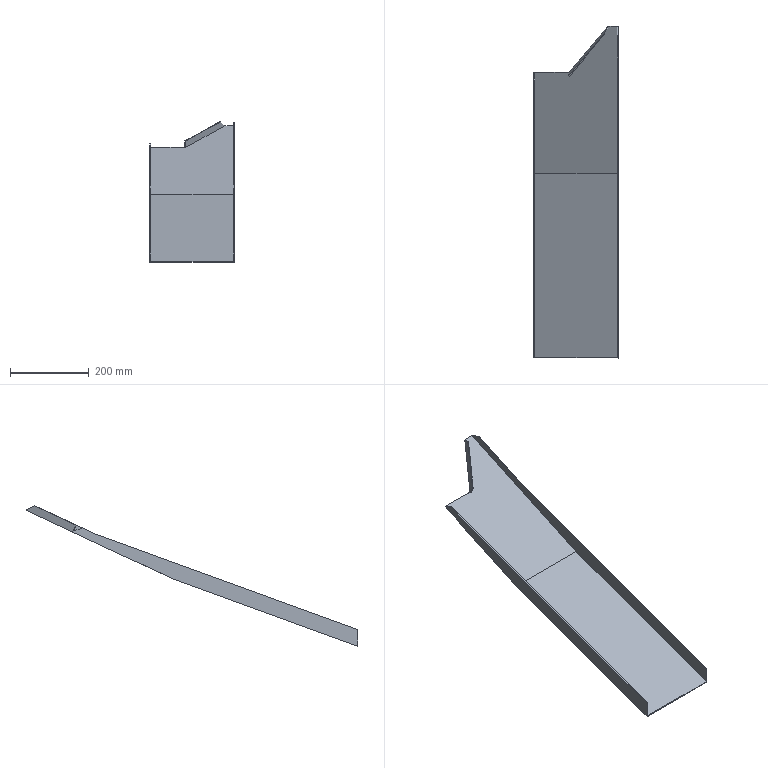Part | NX | features solid 2 | 1 solid | 26 faces | box 215.004 x 843.442 x 357.356 mm | volume 469723 mm3 | plane 26
STEP:
#1=CARTESIAN_POINT('',(-102.,-351.532,-337.023));
#2=VERTEX_POINT('',#1);
#3=CARTESIAN_POINT('',(-313.,-351.532,-337.004));
#4=VERTEX_POINT('',#3);
#5=CARTESIAN_POINT('',(-135.01,-351.532,-337.02));
#6=DIRECTION('',(1.,0.,-0.00008812));
#7=VECTOR('',#6,1000.);
#8=LINE('',#5,#7);
#9=EDGE_CURVE('',#2,#4,#8,.F.);
#10=ORIENTED_EDGE('',*,*,#9,.F.);
#11=CARTESIAN_POINT('',(-101.997,22.596,-162.564));
#12=VERTEX_POINT('',#11);
#13=CARTESIAN_POINT('',(-101.999,-191.108,-262.216));
#14=DIRECTION('',(0.000007217,0.9063,0.4226));
#15=VECTOR('',#14,1000.);
#16=LINE('',#13,#15);
#17=EDGE_CURVE('',#2,#12,#16,.T.);
#18=ORIENTED_EDGE('',*,*,#17,.T.);
#19=CARTESIAN_POINT('',(-126.636,22.592,-162.564));
#20=VERTEX_POINT('',#19);
#21=CARTESIAN_POINT('',(72.152,22.629,-162.564));
#22=DIRECTION('',(-1.,-0.000189,0.));
#23=VECTOR('',#22,1000.);
#24=LINE('',#21,#23);
#25=EDGE_CURVE('',#12,#20,#24,.T.);
#26=ORIENTED_EDGE('',*,*,#25,.T.);
#27=CARTESIAN_POINT('',(-125.044,21.495,-163.076));
#28=VERTEX_POINT('',#27);
#29=CARTESIAN_POINT('',(-18.326,-52.058,-197.383));
#30=DIRECTION('',(0.796,-0.5486,-0.2559));
#31=VECTOR('',#30,1000.);
#32=LINE('',#29,#31);
#33=EDGE_CURVE('',#28,#20,#32,.F.);
#34=ORIENTED_EDGE('',*,*,#33,.F.);
#35=CARTESIAN_POINT('',(-223.923,-96.344,-218.016));
#36=VERTEX_POINT('',#35);
#37=CARTESIAN_POINT('',(-241.722,-117.556,-227.906));
#38=DIRECTION('',(-0.6053,-0.7214,-0.3363));
#39=VECTOR('',#38,1000.);
#40=LINE('',#37,#39);
#41=EDGE_CURVE('',#28,#36,#40,.T.);
#42=ORIENTED_EDGE('',*,*,#41,.T.);
#43=CARTESIAN_POINT('',(-225.515,-95.247,-217.504));
#44=VERTEX_POINT('',#43);
#45=CARTESIAN_POINT('',(-117.204,-169.896,-252.323));
#46=DIRECTION('',(0.796,-0.5486,-0.2559));
#47=VECTOR('',#46,1000.);
#48=LINE('',#45,#47);
#49=EDGE_CURVE('',#44,#36,#48,.T.);
#50=ORIENTED_EDGE('',*,*,#49,.F.);
#51=CARTESIAN_POINT('',(-224.805,-94.402,-217.11));
#52=VERTEX_POINT('',#51);
#53=CARTESIAN_POINT('',(-243.314,-116.459,-227.394));
#54=DIRECTION('',(-0.6053,-0.7214,-0.3363));
#55=VECTOR('',#54,1000.);
#56=LINE('',#53,#55);
#57=EDGE_CURVE('',#52,#44,#56,.T.);
#58=ORIENTED_EDGE('',*,*,#57,.F.);
#59=CARTESIAN_POINT('',(-314.998,-94.419,-217.11));
#60=VERTEX_POINT('',#59);
#61=CARTESIAN_POINT('',(-135.022,-94.385,-217.11));
#62=DIRECTION('',(1.,0.000189,0.));
#63=VECTOR('',#62,1000.);
#64=LINE('',#61,#63);
#65=EDGE_CURVE('',#60,#52,#64,.T.);
#66=ORIENTED_EDGE('',*,*,#65,.F.);
#67=CARTESIAN_POINT('',(-314.998,-95.264,-217.504));
#68=VERTEX_POINT('',#67);
#69=CARTESIAN_POINT('',(-314.999,-191.114,-262.2));
#70=DIRECTION('',(0.000007217,0.9063,0.4226));
#71=VECTOR('',#70,1000.);
#72=LINE('',#69,#71);
#73=EDGE_CURVE('',#60,#68,#72,.F.);
#74=ORIENTED_EDGE('',*,*,#73,.T.);
#75=CARTESIAN_POINT('',(-312.998,-95.264,-217.504));
#76=VERTEX_POINT('',#75);
#77=CARTESIAN_POINT('',(-312.998,-95.264,-217.504));
#78=DIRECTION('',(1.,0.00002832,-0.00007781));
#79=VECTOR('',#78,1000.);
#80=LINE('',#77,#79);
#81=EDGE_CURVE('',#68,#76,#80,.T.);
#82=ORIENTED_EDGE('',*,*,#81,.T.);
#83=CARTESIAN_POINT('',(-312.999,-191.114,-262.2));
#84=DIRECTION('',(-0.000007217,-0.9063,-0.4226));
#85=VECTOR('',#84,1000.);
#86=LINE('',#83,#85);
#87=EDGE_CURVE('',#76,#4,#86,.T.);
#88=ORIENTED_EDGE('',*,*,#87,.T.);
#89=EDGE_LOOP('',(#10,#18,#26,#34,#42,#50,#58,#66,#74,#82,#88));
#90=FACE_BOUND('',#89,.T.);
#91=CARTESIAN_POINT('',(-135.004,-191.109,-262.213));
#92=DIRECTION('',(0.00007986,-0.4226,0.9063));
#93=DIRECTION('',(1.,0.0000177,-0.00007986));
#94=AXIS2_PLACEMENT_3D('',#91,#92,#93);
#95=PLANE('',#94);
#96=ADVANCED_FACE('',(#90),#95,.T.);
#97=CARTESIAN_POINT('',(-315.,-820.,-509.641));
#98=VERTEX_POINT('',#97);
#99=CARTESIAN_POINT('',(-314.997,-820.,-467.074));
#100=VERTEX_POINT('',#99);
#101=CARTESIAN_POINT('',(-315.015,-820.,-699.893));
#102=DIRECTION('',(-0.00007781,0.,-1.));
#103=VECTOR('',#102,1000.);
#104=LINE('',#101,#103);
#105=EDGE_CURVE('',#98,#100,#104,.F.);
#106=ORIENTED_EDGE('',*,*,#105,.F.);
#107=CARTESIAN_POINT('',(-100.,-820.,-509.66));
#108=VERTEX_POINT('',#107);
#109=CARTESIAN_POINT('',(1065.017,-820.,-509.762));
#110=DIRECTION('',(1.,0.,-0.00008812));
#111=VECTOR('',#110,1000.);
#112=LINE('',#109,#111);
#113=EDGE_CURVE('',#108,#98,#112,.F.);
#114=ORIENTED_EDGE('',*,*,#113,.F.);
#115=CARTESIAN_POINT('',(-99.997,-820.,-467.093));
#116=VERTEX_POINT('',#115);
#117=CARTESIAN_POINT('',(-100.015,-820.,-699.909));
#118=DIRECTION('',(-0.00007781,0.,-1.));
#119=VECTOR('',#118,1000.);
#120=LINE('',#117,#119);
#121=EDGE_CURVE('',#116,#108,#120,.T.);
#122=ORIENTED_EDGE('',*,*,#121,.F.);
#123=CARTESIAN_POINT('',(-101.997,-820.,-467.092));
#124=VERTEX_POINT('',#123);
#125=CARTESIAN_POINT('',(1065.021,-820.,-467.195));
#126=DIRECTION('',(-1.,0.,0.00008812));
#127=VECTOR('',#126,1000.);
#128=LINE('',#125,#127);
#129=EDGE_CURVE('',#124,#116,#128,.F.);
#130=ORIENTED_EDGE('',*,*,#129,.F.);
#131=CARTESIAN_POINT('',(-102.,-820.,-507.531));
#132=VERTEX_POINT('',#131);
#133=CARTESIAN_POINT('',(-101.973,-820.,-164.376));
#134=DIRECTION('',(0.00007781,0.,1.));
#135=VECTOR('',#134,1000.);
#136=LINE('',#133,#135);
#137=EDGE_CURVE('',#132,#124,#136,.T.);
#138=ORIENTED_EDGE('',*,*,#137,.F.);
#139=CARTESIAN_POINT('',(-313.,-820.,-507.513));
#140=VERTEX_POINT('',#139);
#141=CARTESIAN_POINT('',(1065.017,-820.,-507.634));
#142=DIRECTION('',(1.,0.,-0.00008812));
#143=VECTOR('',#142,1000.);
#144=LINE('',#141,#143);
#145=EDGE_CURVE('',#132,#140,#144,.F.);
#146=ORIENTED_EDGE('',*,*,#145,.T.);
#147=CARTESIAN_POINT('',(-312.997,-820.,-467.074));
#148=VERTEX_POINT('',#147);
#149=CARTESIAN_POINT('',(-312.987,-820.,-338.854));
#150=DIRECTION('',(-0.00007781,0.,-1.));
#151=VECTOR('',#150,1000.);
#152=LINE('',#149,#151);
#153=EDGE_CURVE('',#148,#140,#152,.T.);
#154=ORIENTED_EDGE('',*,*,#153,.F.);
#155=CARTESIAN_POINT('',(-315.011,-820.,-467.074));
#156=DIRECTION('',(-1.,0.,0.00008812));
#157=VECTOR('',#156,1000.);
#158=LINE('',#155,#157);
#159=EDGE_CURVE('',#100,#148,#158,.F.);
#160=ORIENTED_EDGE('',*,*,#159,.F.);
#161=EDGE_LOOP('',(#106,#114,#122,#130,#138,#146,#154,#160));
#162=FACE_BOUND('',#161,.T.);
#163=CARTESIAN_POINT('',(1065.,-820.,-700.));
#164=DIRECTION('',(0.,1.,0.));
#165=DIRECTION('',(-1.,0.,0.));
#166=AXIS2_PLACEMENT_3D('',#163,#164,#165);
#167=PLANE('',#166);
#168=ADVANCED_FACE('',(#162),#167,.F.);
#169=ORIENTED_EDGE('',*,*,#145,.F.);
#170=CARTESIAN_POINT('',(-102.,-184.87,-276.363));
#171=DIRECTION('',(0.,0.9397,0.342));
#172=VECTOR('',#171,1000.);
#173=LINE('',#170,#172);
#174=EDGE_CURVE('',#132,#2,#173,.T.);
#175=ORIENTED_EDGE('',*,*,#174,.T.);
#176=ORIENTED_EDGE('',*,*,#9,.T.);
#177=CARTESIAN_POINT('',(-313.,-184.876,-276.346));
#178=DIRECTION('',(0.,-0.9397,-0.342));
#179=VECTOR('',#178,1000.);
#180=LINE('',#177,#179);
#181=EDGE_CURVE('',#4,#140,#180,.T.);
#182=ORIENTED_EDGE('',*,*,#181,.T.);
#183=EDGE_LOOP('',(#169,#175,#176,#182));
#184=FACE_BOUND('',#183,.T.);
#185=CARTESIAN_POINT('',(-135.005,-184.871,-276.36));
#186=DIRECTION('',(0.0000828,-0.342,0.9397));
#187=DIRECTION('',(1.,0.00001836,-0.00008143));
#188=AXIS2_PLACEMENT_3D('',#185,#186,#187);
#189=PLANE('',#188);
#190=ADVANCED_FACE('',(#184),#189,.T.);
#191=CARTESIAN_POINT('',(-101.997,23.442,-164.376));
#192=VERTEX_POINT('',#191);
#193=CARTESIAN_POINT('',(-101.997,22.596,-162.563));
#194=DIRECTION('',(0.00008249,-0.4226,0.9063));
#195=VECTOR('',#194,1000.);
#196=LINE('',#193,#195);
#197=EDGE_CURVE('',#192,#12,#196,.T.);
#198=ORIENTED_EDGE('',*,*,#197,.F.);
#199=CARTESIAN_POINT('',(-126.636,23.437,-164.376));
#200=VERTEX_POINT('',#199);
#201=CARTESIAN_POINT('',(72.152,23.474,-164.376));
#202=DIRECTION('',(-1.,-0.000189,0.));
#203=VECTOR('',#202,1000.);
#204=LINE('',#201,#203);
#205=EDGE_CURVE('',#192,#200,#204,.T.);
#206=ORIENTED_EDGE('',*,*,#205,.T.);
#207=CARTESIAN_POINT('',(-126.636,22.592,-162.564));
#208=DIRECTION('',(-0.00007986,0.4226,-0.9063));
#209=VECTOR('',#208,1000.);
#210=LINE('',#207,#209);
#211=EDGE_CURVE('',#200,#20,#210,.F.);
#212=ORIENTED_EDGE('',*,*,#211,.T.);
#213=ORIENTED_EDGE('',*,*,#25,.F.);
#214=EDGE_LOOP('',(#198,#206,#212,#213));
#215=FACE_BOUND('',#214,.T.);
#216=CARTESIAN_POINT('',(72.152,22.629,-162.564));
#217=DIRECTION('',(0.0001713,-0.9063,-0.4226));
#218=DIRECTION('',(0.,0.4226,-0.9063));
#219=AXIS2_PLACEMENT_3D('',#216,#217,#218);
#220=PLANE('',#219);
#221=ADVANCED_FACE('',(#215),#220,.F.);
#222=CARTESIAN_POINT('',(-102.,-350.766,-338.872));
#223=VERTEX_POINT('',#222);
#224=CARTESIAN_POINT('',(-100.,-350.766,-338.873));
#225=VERTEX_POINT('',#224);
#226=CARTESIAN_POINT('',(-100.,-350.766,-338.873));
#227=CARTESIAN_POINT('',(-100.667,-350.766,-338.872));
#228=CARTESIAN_POINT('',(-101.333,-350.766,-338.872));
#229=CARTESIAN_POINT('',(-102.,-350.766,-338.872));
#230=B_SPLINE_CURVE_WITH_KNOTS('',3,(#226,#227,#228,#229),.UNSPECIFIED.,.F.,.F.,(4,4),(0.,1.),.UNSPECIFIED.);
#231=EDGE_CURVE('',#223,#225,#230,.F.);
#232=ORIENTED_EDGE('',*,*,#231,.F.);
#233=CARTESIAN_POINT('',(-313.,-350.766,-338.854));
#234=VERTEX_POINT('',#233);
#235=CARTESIAN_POINT('',(-135.01,-350.766,-338.869));
#236=DIRECTION('',(-1.,0.,0.00008812));
#237=VECTOR('',#236,1000.);
#238=LINE('',#235,#237);
#239=EDGE_CURVE('',#234,#223,#238,.F.);
#240=ORIENTED_EDGE('',*,*,#239,.F.);
#241=CARTESIAN_POINT('',(-315.,-350.766,-338.854));
#242=VERTEX_POINT('',#241);
#243=CARTESIAN_POINT('',(-315.,-350.766,-338.854));
#244=CARTESIAN_POINT('',(-314.333,-350.766,-338.854));
#245=CARTESIAN_POINT('',(-313.667,-350.766,-338.854));
#246=CARTESIAN_POINT('',(-313.,-350.766,-338.854));
#247=B_SPLINE_CURVE_WITH_KNOTS('',3,(#243,#244,#245,#246),.UNSPECIFIED.,.F.,.F.,(4,4),(0.,1.),.UNSPECIFIED.);
#248=EDGE_CURVE('',#242,#234,#247,.T.);
#249=ORIENTED_EDGE('',*,*,#248,.F.);
#250=CARTESIAN_POINT('',(-314.998,-94.419,-219.317));
#251=VERTEX_POINT('',#250);
#252=CARTESIAN_POINT('',(-314.999,-190.268,-264.012));
#253=DIRECTION('',(0.000007217,0.9063,0.4226));
#254=VECTOR('',#253,1000.);
#255=LINE('',#252,#254);
#256=EDGE_CURVE('',#251,#242,#255,.F.);
#257=ORIENTED_EDGE('',*,*,#256,.F.);
#258=CARTESIAN_POINT('',(-225.515,-94.402,-219.317));
#259=VERTEX_POINT('',#258);
#260=CARTESIAN_POINT('',(-135.022,-94.385,-219.317));
#261=DIRECTION('',(1.,0.000189,0.));
#262=VECTOR('',#261,1000.);
#263=LINE('',#260,#262);
#264=EDGE_CURVE('',#251,#259,#263,.T.);
#265=ORIENTED_EDGE('',*,*,#264,.T.);
#266=CARTESIAN_POINT('',(-243.314,-115.614,-229.207));
#267=DIRECTION('',(-0.6053,-0.7214,-0.3363));
#268=VECTOR('',#267,1000.);
#269=LINE('',#266,#268);
#270=EDGE_CURVE('',#200,#259,#269,.T.);
#271=ORIENTED_EDGE('',*,*,#270,.F.);
#272=ORIENTED_EDGE('',*,*,#205,.F.);
#273=CARTESIAN_POINT('',(-99.997,23.442,-164.376));
#274=VERTEX_POINT('',#273);
#275=CARTESIAN_POINT('',(72.152,23.474,-164.376));
#276=DIRECTION('',(-1.,-0.000189,0.));
#277=VECTOR('',#276,1000.);
#278=LINE('',#275,#277);
#279=EDGE_CURVE('',#274,#192,#278,.T.);
#280=ORIENTED_EDGE('',*,*,#279,.F.);
#281=CARTESIAN_POINT('',(-99.999,-190.558,-264.166));
#282=DIRECTION('',(-0.000007217,-0.9063,-0.4226));
#283=VECTOR('',#282,1000.);
#284=LINE('',#281,#283);
#285=EDGE_CURVE('',#274,#225,#284,.T.);
#286=ORIENTED_EDGE('',*,*,#285,.T.);
#287=EDGE_LOOP('',(#232,#240,#249,#257,#265,#271,#272,#280,#286));
#288=FACE_BOUND('',#287,.T.);
#289=CARTESIAN_POINT('',(-135.004,-190.263,-264.026));
#290=DIRECTION('',(0.00007986,-0.4226,0.9063));
#291=DIRECTION('',(1.,0.0000177,-0.00007986));
#292=AXIS2_PLACEMENT_3D('',#289,#290,#291);
#293=PLANE('',#292);
#294=ADVANCED_FACE('',(#288),#293,.F.);
#295=CARTESIAN_POINT('',(-126.636,22.592,-162.564));
#296=VERTEX_POINT('',#295);
#297=CARTESIAN_POINT('',(-126.636,23.437,-164.376));
#298=DIRECTION('',(0.,-0.4226,0.9063));
#299=VECTOR('',#298,1000.);
#300=LINE('',#297,#299);
#301=EDGE_CURVE('',#200,#296,#300,.T.);
#302=ORIENTED_EDGE('',*,*,#301,.F.);
#303=ORIENTED_EDGE('',*,*,#270,.T.);
#304=CARTESIAN_POINT('',(-200.25,-94.397,-140.71));
#305=DIRECTION('',(0.306,0.00005782,0.952));
#306=VECTOR('',#305,1000.);
#307=LINE('',#304,#306);
#308=EDGE_CURVE('',#259,#52,#307,.T.);
#309=ORIENTED_EDGE('',*,*,#308,.T.);
#310=ORIENTED_EDGE('',*,*,#57,.T.);
#311=CARTESIAN_POINT('',(-225.515,-102.853,-201.19));
#312=VERTEX_POINT('',#311);
#313=CARTESIAN_POINT('',(-225.515,-94.402,-219.317));
#314=DIRECTION('',(0.,-0.4226,0.9063));
#315=VECTOR('',#314,1000.);
#316=LINE('',#313,#315);
#317=EDGE_CURVE('',#44,#312,#316,.T.);
#318=ORIENTED_EDGE('',*,*,#317,.T.);
#319=CARTESIAN_POINT('',(-137.532,2.,-152.304));
#320=VERTEX_POINT('',#319);
#321=CARTESIAN_POINT('',(-126.636,14.986,-146.25));
#322=DIRECTION('',(-0.6053,-0.7214,-0.3363));
#323=VECTOR('',#322,1000.);
#324=LINE('',#321,#323);
#325=EDGE_CURVE('',#320,#312,#324,.T.);
#326=ORIENTED_EDGE('',*,*,#325,.F.);
#327=CARTESIAN_POINT('',(-126.031,23.736,-163.134));
#328=DIRECTION('',(-0.428,-0.8089,0.403));
#329=VECTOR('',#328,1000.);
#330=LINE('',#327,#329);
#331=EDGE_CURVE('',#320,#296,#330,.F.);
#332=ORIENTED_EDGE('',*,*,#331,.T.);
#333=EDGE_LOOP('',(#302,#303,#309,#310,#318,#326,#332));
#334=FACE_BOUND('',#333,.T.);
#335=CARTESIAN_POINT('',(-126.636,23.437,-164.376));
#336=DIRECTION('',(-0.796,0.5486,0.2558));
#337=DIRECTION('',(-0.5675,-0.8234,0.));
#338=AXIS2_PLACEMENT_3D('',#335,#336,#337);
#339=PLANE('',#338);
#340=ADVANCED_FACE('',(#334),#339,.T.);
#341=ORIENTED_EDGE('',*,*,#121,.T.);
#342=CARTESIAN_POINT('',(-100.,-184.186,-278.242));
#343=DIRECTION('',(0.,0.9397,0.342));
#344=VECTOR('',#343,1000.);
#345=LINE('',#342,#344);
#346=EDGE_CURVE('',#225,#108,#345,.F.);
#347=ORIENTED_EDGE('',*,*,#346,.F.);
#348=ORIENTED_EDGE('',*,*,#285,.F.);
#349=CARTESIAN_POINT('',(-99.997,22.597,-162.564));
#350=VERTEX_POINT('',#349);
#351=CARTESIAN_POINT('',(-99.998,29.129,-176.573));
#352=DIRECTION('',(-0.00008249,0.4226,-0.9063));
#353=VECTOR('',#352,1000.);
#354=LINE('',#351,#353);
#355=EDGE_CURVE('',#350,#274,#354,.T.);
#356=ORIENTED_EDGE('',*,*,#355,.F.);
#357=CARTESIAN_POINT('',(-99.996,-1.324,-153.857));
#358=VERTEX_POINT('',#357);
#359=CARTESIAN_POINT('',(-99.996,-1.324,-153.857));
#360=DIRECTION('',(0.00005322,-0.9397,0.342));
#361=VECTOR('',#360,1000.);
#362=LINE('',#359,#361);
#363=EDGE_CURVE('',#350,#358,#362,.T.);
#364=ORIENTED_EDGE('',*,*,#363,.T.);
#365=CARTESIAN_POINT('',(-99.997,-150.453,-223.397));
#366=VERTEX_POINT('',#365);
#367=CARTESIAN_POINT('',(-99.995,14.99,-146.25));
#368=DIRECTION('',(-0.000007217,-0.9063,-0.4226));
#369=VECTOR('',#368,1000.);
#370=LINE('',#367,#369);
#371=EDGE_CURVE('',#358,#366,#370,.T.);
#372=ORIENTED_EDGE('',*,*,#371,.T.);
#373=CARTESIAN_POINT('',(-99.997,-364.447,-301.285));
#374=DIRECTION('',(0.,-0.9397,-0.342));
#375=VECTOR('',#374,1000.);
#376=LINE('',#373,#375);
#377=EDGE_CURVE('',#366,#116,#376,.T.);
#378=ORIENTED_EDGE('',*,*,#377,.T.);
#379=EDGE_LOOP('',(#341,#347,#348,#356,#364,#372,#378));
#380=FACE_BOUND('',#379,.T.);
#381=CARTESIAN_POINT('',(-100.,-184.87,-276.363));
#382=DIRECTION('',(1.,0.00002832,-0.00007781));
#383=DIRECTION('',(-0.00007781,0.,-1.));
#384=AXIS2_PLACEMENT_3D('',#381,#382,#383);
#385=PLANE('',#384);
#386=ADVANCED_FACE('',(#380),#385,.T.);
#387=ORIENTED_EDGE('',*,*,#65,.T.);
#388=ORIENTED_EDGE('',*,*,#308,.F.);
#389=ORIENTED_EDGE('',*,*,#264,.F.);
#390=CARTESIAN_POINT('',(-314.993,-94.419,-153.115));
#391=DIRECTION('',(0.00007781,0.000000015,1.));
#392=VECTOR('',#391,1000.);
#393=LINE('',#390,#392);
#394=EDGE_CURVE('',#60,#251,#393,.F.);
#395=ORIENTED_EDGE('',*,*,#394,.F.);
#396=EDGE_LOOP('',(#387,#388,#389,#395));
#397=FACE_BOUND('',#396,.T.);
#398=CARTESIAN_POINT('',(-325.,-94.421,-153.114));
#399=DIRECTION('',(0.000189,-1.,0.));
#400=DIRECTION('',(1.,0.000189,0.));
#401=AXIS2_PLACEMENT_3D('',#398,#399,#400);
#402=PLANE('',#401);
#403=ADVANCED_FACE('',(#397),#402,.F.);
#404=CARTESIAN_POINT('',(-314.996,-119.185,-208.798));
#405=VERTEX_POINT('',#404);
#406=CARTESIAN_POINT('',(-314.998,-95.264,-217.504));
#407=DIRECTION('',(0.00005322,-0.9397,0.342));
#408=VECTOR('',#407,1000.);
#409=LINE('',#406,#408);
#410=EDGE_CURVE('',#405,#68,#409,.F.);
#411=ORIENTED_EDGE('',*,*,#410,.T.);
#412=ORIENTED_EDGE('',*,*,#73,.F.);
#413=ORIENTED_EDGE('',*,*,#394,.T.);
#414=ORIENTED_EDGE('',*,*,#256,.T.);
#415=CARTESIAN_POINT('',(-315.,-184.192,-278.226));
#416=DIRECTION('',(0.,0.9397,0.342));
#417=VECTOR('',#416,1000.);
#418=LINE('',#415,#417);
#419=EDGE_CURVE('',#242,#98,#418,.F.);
#420=ORIENTED_EDGE('',*,*,#419,.T.);
#421=ORIENTED_EDGE('',*,*,#105,.T.);
#422=CARTESIAN_POINT('',(-314.997,-150.453,-223.378));
#423=VERTEX_POINT('',#422);
#424=CARTESIAN_POINT('',(-314.997,-197.873,-240.638));
#425=DIRECTION('',(0.,-0.9397,-0.342));
#426=VECTOR('',#425,1000.);
#427=LINE('',#424,#426);
#428=EDGE_CURVE('',#423,#100,#427,.T.);
#429=ORIENTED_EDGE('',*,*,#428,.F.);
#430=CARTESIAN_POINT('',(-314.996,-102.871,-201.191));
#431=DIRECTION('',(-0.000007217,-0.9063,-0.4226));
#432=VECTOR('',#431,1000.);
#433=LINE('',#430,#432);
#434=EDGE_CURVE('',#405,#423,#433,.T.);
#435=ORIENTED_EDGE('',*,*,#434,.F.);
#436=EDGE_LOOP('',(#411,#412,#413,#414,#420,#421,#429,#435));
#437=FACE_BOUND('',#436,.T.);
#438=CARTESIAN_POINT('',(-315.,-184.876,-276.346));
#439=DIRECTION('',(1.,0.00002832,-0.00007781));
#440=DIRECTION('',(-0.00007781,0.,-1.));
#441=AXIS2_PLACEMENT_3D('',#438,#439,#440);
#442=PLANE('',#441);
#443=ADVANCED_FACE('',(#437),#442,.F.);
#444=ORIENTED_EDGE('',*,*,#346,.T.);
#445=ORIENTED_EDGE('',*,*,#113,.T.);
#446=ORIENTED_EDGE('',*,*,#419,.F.);
#447=ORIENTED_EDGE('',*,*,#248,.T.);
#448=ORIENTED_EDGE('',*,*,#239,.T.);
#449=ORIENTED_EDGE('',*,*,#231,.T.);
#450=EDGE_LOOP('',(#444,#445,#446,#447,#448,#449));
#451=FACE_BOUND('',#450,.T.);
#452=CARTESIAN_POINT('',(-135.005,-184.187,-278.24));
#453=DIRECTION('',(0.0000828,-0.342,0.9397));
#454=DIRECTION('',(1.,0.00001836,-0.00008143));
#455=AXIS2_PLACEMENT_3D('',#452,#453,#454);
#456=PLANE('',#455);
#457=ADVANCED_FACE('',(#451),#456,.F.);
#458=ORIENTED_EDGE('',*,*,#211,.F.);
#459=ORIENTED_EDGE('',*,*,#301,.T.);
#460=CARTESIAN_POINT('',(-126.636,22.592,-162.564));
#461=DIRECTION('',(-0.796,0.5486,0.2558));
#462=VECTOR('',#461,1000.);
#463=LINE('',#460,#462);
#464=EDGE_CURVE('',#296,#20,#463,.F.);
#465=ORIENTED_EDGE('',*,*,#464,.T.);
#466=EDGE_LOOP('',(#458,#459,#465));
#467=FACE_BOUND('',#466,.T.);
#468=CARTESIAN_POINT('',(-126.636,23.437,-164.376));
#469=DIRECTION('',(-0.6053,-0.7214,-0.3363));
#470=DIRECTION('',(0.,-0.4226,0.9063));
#471=AXIS2_PLACEMENT_3D('',#468,#469,#470);
#472=PLANE('',#471);
#473=ADVANCED_FACE('',(#467),#472,.F.);
#474=CARTESIAN_POINT('',(-125.044,21.494,-163.075));
#475=VERTEX_POINT('',#474);
#476=CARTESIAN_POINT('',(-125.044,22.34,-164.888));
#477=DIRECTION('',(0.,-0.4226,0.9063));
#478=VECTOR('',#477,1000.);
#479=LINE('',#476,#478);
#480=EDGE_CURVE('',#28,#475,#479,.T.);
#481=ORIENTED_EDGE('',*,*,#480,.F.);
#482=ORIENTED_EDGE('',*,*,#33,.T.);
#483=CARTESIAN_POINT('',(-126.636,22.592,-162.564));
#484=DIRECTION('',(-0.796,0.5486,0.2558));
#485=VECTOR('',#484,1000.);
#486=LINE('',#483,#485);
#487=EDGE_CURVE('',#20,#475,#486,.F.);
#488=ORIENTED_EDGE('',*,*,#487,.T.);
#489=EDGE_LOOP('',(#481,#482,#488));
#490=FACE_BOUND('',#489,.T.);
#491=CARTESIAN_POINT('',(-126.636,23.437,-164.376));
#492=DIRECTION('',(-0.6053,-0.7214,-0.3363));
#493=DIRECTION('',(0.,-0.4226,0.9063));
#494=AXIS2_PLACEMENT_3D('',#491,#492,#493);
#495=PLANE('',#494);
#496=ADVANCED_FACE('',(#490),#495,.F.);
#497=CARTESIAN_POINT('',(-135.94,0.9029,-152.816));
#498=VERTEX_POINT('',#497);
#499=CARTESIAN_POINT('',(-223.923,-103.95,-201.702));
#500=VERTEX_POINT('',#499);
#501=CARTESIAN_POINT('',(-125.044,13.888,-146.761));
#502=DIRECTION('',(-0.6053,-0.7214,-0.3363));
#503=VECTOR('',#502,1000.);
#504=LINE('',#501,#503);
#505=EDGE_CURVE('',#498,#500,#504,.T.);
#506=ORIENTED_EDGE('',*,*,#505,.F.);
#507=CARTESIAN_POINT('',(-137.532,2.,-152.304));
#508=DIRECTION('',(0.796,-0.5486,-0.2558));
#509=VECTOR('',#508,1000.);
#510=LINE('',#507,#509);
#511=EDGE_CURVE('',#498,#320,#510,.F.);
#512=ORIENTED_EDGE('',*,*,#511,.T.);
#513=ORIENTED_EDGE('',*,*,#325,.T.);
#514=CARTESIAN_POINT('',(-225.515,-102.853,-201.19));
#515=DIRECTION('',(0.796,-0.5486,-0.2558));
#516=VECTOR('',#515,1000.);
#517=LINE('',#514,#516);
#518=EDGE_CURVE('',#312,#500,#517,.T.);
#519=ORIENTED_EDGE('',*,*,#518,.T.);
#520=EDGE_LOOP('',(#506,#512,#513,#519));
#521=FACE_BOUND('',#520,.T.);
#522=CARTESIAN_POINT('',(-126.636,14.986,-146.25));
#523=DIRECTION('',(0.,0.4226,-0.9063));
#524=DIRECTION('',(-0.6053,-0.7214,-0.3363));
#525=AXIS2_PLACEMENT_3D('',#522,#523,#524);
#526=PLANE('',#525);
#527=ADVANCED_FACE('',(#521),#526,.F.);
#528=ORIENTED_EDGE('',*,*,#41,.F.);
#529=ORIENTED_EDGE('',*,*,#480,.T.);
#530=CARTESIAN_POINT('',(-125.044,21.494,-163.075));
#531=DIRECTION('',(0.428,0.8089,-0.403));
#532=VECTOR('',#531,1000.);
#533=LINE('',#530,#532);
#534=EDGE_CURVE('',#475,#498,#533,.F.);
#535=ORIENTED_EDGE('',*,*,#534,.T.);
#536=ORIENTED_EDGE('',*,*,#505,.T.);
#537=CARTESIAN_POINT('',(-223.923,-95.499,-219.828));
#538=DIRECTION('',(0.,-0.4226,0.9063));
#539=VECTOR('',#538,1000.);
#540=LINE('',#537,#539);
#541=EDGE_CURVE('',#36,#500,#540,.T.);
#542=ORIENTED_EDGE('',*,*,#541,.F.);
#543=EDGE_LOOP('',(#528,#529,#535,#536,#542));
#544=FACE_BOUND('',#543,.T.);
#545=CARTESIAN_POINT('',(-125.044,22.34,-164.888));
#546=DIRECTION('',(-0.796,0.5486,0.2558));
#547=DIRECTION('',(-0.5675,-0.8234,0.));
#548=AXIS2_PLACEMENT_3D('',#545,#546,#547);
#549=PLANE('',#548);
#550=ADVANCED_FACE('',(#544),#549,.F.);
#551=ORIENTED_EDGE('',*,*,#317,.F.);
#552=ORIENTED_EDGE('',*,*,#49,.T.);
#553=ORIENTED_EDGE('',*,*,#541,.T.);
#554=ORIENTED_EDGE('',*,*,#518,.F.);
#555=EDGE_LOOP('',(#551,#552,#553,#554));
#556=FACE_BOUND('',#555,.T.);
#557=CARTESIAN_POINT('',(-225.515,-94.402,-219.317));
#558=DIRECTION('',(-0.6053,-0.7214,-0.3363));
#559=DIRECTION('',(0.,-0.4226,0.9063));
#560=AXIS2_PLACEMENT_3D('',#557,#558,#559);
#561=PLANE('',#560);
#562=ADVANCED_FACE('',(#556),#561,.T.);
#563=ORIENTED_EDGE('',*,*,#331,.F.);
#564=ORIENTED_EDGE('',*,*,#511,.F.);
#565=ORIENTED_EDGE('',*,*,#534,.F.);
#566=ORIENTED_EDGE('',*,*,#487,.F.);
#567=ORIENTED_EDGE('',*,*,#464,.F.);
#568=EDGE_LOOP('',(#563,#564,#565,#566,#567));
#569=FACE_BOUND('',#568,.T.);
#570=CARTESIAN_POINT('',(-126.636,22.592,-162.564));
#571=DIRECTION('',(-0.428,-0.2113,-0.8787));
#572=DIRECTION('',(-0.899,0.,0.4379));
#573=AXIS2_PLACEMENT_3D('',#570,#571,#572);
#574=PLANE('',#573);
#575=ADVANCED_FACE('',(#569),#574,.F.);
#576=ORIENTED_EDGE('',*,*,#87,.F.);
#577=CARTESIAN_POINT('',(-312.996,-119.185,-208.798));
#578=VERTEX_POINT('',#577);
#579=CARTESIAN_POINT('',(-312.998,-95.264,-217.504));
#580=DIRECTION('',(0.00005322,-0.9397,0.342));
#581=VECTOR('',#580,1000.);
#582=LINE('',#579,#581);
#583=EDGE_CURVE('',#76,#578,#582,.T.);
#584=ORIENTED_EDGE('',*,*,#583,.T.);
#585=CARTESIAN_POINT('',(-312.997,-150.453,-223.379));
#586=VERTEX_POINT('',#585);
#587=CARTESIAN_POINT('',(-312.996,-102.871,-201.191));
#588=DIRECTION('',(-0.000007217,-0.9063,-0.4226));
#589=VECTOR('',#588,1000.);
#590=LINE('',#587,#589);
#591=EDGE_CURVE('',#578,#586,#590,.T.);
#592=ORIENTED_EDGE('',*,*,#591,.T.);
#593=CARTESIAN_POINT('',(-312.997,-364.447,-301.266));
#594=DIRECTION('',(0.,-0.9397,-0.342));
#595=VECTOR('',#594,1000.);
#596=LINE('',#593,#595);
#597=EDGE_CURVE('',#586,#148,#596,.T.);
#598=ORIENTED_EDGE('',*,*,#597,.T.);
#599=ORIENTED_EDGE('',*,*,#153,.T.);
#600=ORIENTED_EDGE('',*,*,#181,.F.);
#601=EDGE_LOOP('',(#576,#584,#592,#598,#599,#600));
#602=FACE_BOUND('',#601,.T.);
#603=CARTESIAN_POINT('',(-313.,-350.766,-338.854));
#604=DIRECTION('',(-1.,-0.00002832,0.00007781));
#605=DIRECTION('',(0.,-0.9397,-0.342));
#606=AXIS2_PLACEMENT_3D('',#603,#604,#605);
#607=PLANE('',#606);
#608=ADVANCED_FACE('',(#602),#607,.F.);
#609=ORIENTED_EDGE('',*,*,#591,.F.);
#610=CARTESIAN_POINT('',(-314.996,-119.185,-208.798));
#611=DIRECTION('',(-1.,-0.00002832,0.00007781));
#612=VECTOR('',#611,1000.);
#613=LINE('',#610,#612);
#614=EDGE_CURVE('',#578,#405,#613,.T.);
#615=ORIENTED_EDGE('',*,*,#614,.T.);
#616=ORIENTED_EDGE('',*,*,#434,.T.);
#617=CARTESIAN_POINT('',(-314.997,-150.453,-223.378));
#618=DIRECTION('',(1.,0.00002832,-0.00007781));
#619=VECTOR('',#618,1000.);
#620=LINE('',#617,#619);
#621=EDGE_CURVE('',#423,#586,#620,.T.);
#622=ORIENTED_EDGE('',*,*,#621,.T.);
#623=EDGE_LOOP('',(#609,#615,#616,#622));
#624=FACE_BOUND('',#623,.T.);
#625=CARTESIAN_POINT('',(-314.996,-102.871,-201.191));
#626=DIRECTION('',(0.00008249,-0.4226,0.9063));
#627=DIRECTION('',(0.,-0.9063,-0.4226));
#628=AXIS2_PLACEMENT_3D('',#625,#626,#627);
#629=PLANE('',#628);
#630=ADVANCED_FACE('',(#624),#629,.T.);
#631=ORIENTED_EDGE('',*,*,#428,.T.);
#632=ORIENTED_EDGE('',*,*,#159,.T.);
#633=ORIENTED_EDGE('',*,*,#597,.F.);
#634=ORIENTED_EDGE('',*,*,#621,.F.);
#635=EDGE_LOOP('',(#631,#632,#633,#634));
#636=FACE_BOUND('',#635,.T.);
#637=CARTESIAN_POINT('',(-314.997,-364.447,-301.266));
#638=DIRECTION('',(0.0000828,-0.342,0.9397));
#639=DIRECTION('',(0.,-0.9397,-0.342));
#640=AXIS2_PLACEMENT_3D('',#637,#638,#639);
#641=PLANE('',#640);
#642=ADVANCED_FACE('',(#636),#641,.T.);
#643=ORIENTED_EDGE('',*,*,#410,.F.);
#644=ORIENTED_EDGE('',*,*,#614,.F.);
#645=ORIENTED_EDGE('',*,*,#583,.F.);
#646=ORIENTED_EDGE('',*,*,#81,.F.);
#647=EDGE_LOOP('',(#643,#644,#645,#646));
#648=FACE_BOUND('',#647,.T.);
#649=CARTESIAN_POINT('',(-314.998,-95.264,-217.504));
#650=DIRECTION('',(0.00006343,0.342,0.9397));
#651=DIRECTION('',(0.,-0.9397,0.342));
#652=AXIS2_PLACEMENT_3D('',#649,#650,#651);
#653=PLANE('',#652);
#654=ADVANCED_FACE('',(#648),#653,.T.);
#655=ORIENTED_EDGE('',*,*,#279,.T.);
#656=CARTESIAN_POINT('',(-101.997,23.442,-164.376));
#657=VERTEX_POINT('',#656);
#658=CARTESIAN_POINT('',(-101.997,23.442,-164.376));
#659=DIRECTION('',(-0.000007217,-0.9063,-0.4226));
#660=VECTOR('',#659,1000.);
#661=LINE('',#658,#660);
#662=EDGE_CURVE('',#657,#192,#661,.T.);
#663=ORIENTED_EDGE('',*,*,#662,.F.);
#664=CARTESIAN_POINT('',(-99.997,23.442,-164.376));
#665=DIRECTION('',(-1.,-0.00002832,0.00007781));
#666=VECTOR('',#665,1000.);
#667=LINE('',#664,#666);
#668=EDGE_CURVE('',#274,#657,#667,.T.);
#669=ORIENTED_EDGE('',*,*,#668,.F.);
#670=EDGE_LOOP('',(#655,#663,#669));
#671=FACE_BOUND('',#670,.T.);
#672=CARTESIAN_POINT('',(-99.997,23.442,-164.376));
#673=DIRECTION('',(-0.00008249,0.4226,-0.9063));
#674=DIRECTION('',(0.,0.9063,0.4226));
#675=AXIS2_PLACEMENT_3D('',#672,#673,#674);
#676=PLANE('',#675);
#677=ADVANCED_FACE('',(#671),#676,.T.);
#678=CARTESIAN_POINT('',(-101.997,22.597,-162.564));
#679=VERTEX_POINT('',#678);
#680=CARTESIAN_POINT('',(-101.997,23.442,-164.376));
#681=DIRECTION('',(-0.00008249,0.4226,-0.9063));
#682=VECTOR('',#681,1000.);
#683=LINE('',#680,#682);
#684=EDGE_CURVE('',#657,#679,#683,.F.);
#685=ORIENTED_EDGE('',*,*,#684,.T.);
#686=CARTESIAN_POINT('',(-99.997,22.597,-162.564));
#687=DIRECTION('',(1.,0.00002832,-0.00007781));
#688=VECTOR('',#687,1000.);
#689=LINE('',#686,#688);
#690=EDGE_CURVE('',#679,#350,#689,.T.);
#691=ORIENTED_EDGE('',*,*,#690,.T.);
#692=ORIENTED_EDGE('',*,*,#355,.T.);
#693=ORIENTED_EDGE('',*,*,#668,.T.);
#694=EDGE_LOOP('',(#685,#691,#692,#693));
#695=FACE_BOUND('',#694,.T.);
#696=CARTESIAN_POINT('',(-99.997,23.442,-164.376));
#697=DIRECTION('',(-0.000007217,-0.9063,-0.4226));
#698=DIRECTION('',(-1.,-0.00002832,0.00007781));
#699=AXIS2_PLACEMENT_3D('',#696,#697,#698);
#700=PLANE('',#699);
#701=ADVANCED_FACE('',(#695),#700,.F.);
#702=ORIENTED_EDGE('',*,*,#174,.F.);
#703=ORIENTED_EDGE('',*,*,#137,.T.);
#704=CARTESIAN_POINT('',(-101.997,-150.453,-223.397));
#705=VERTEX_POINT('',#704);
#706=CARTESIAN_POINT('',(-101.997,-364.447,-301.285));
#707=DIRECTION('',(0.,-0.9397,-0.342));
#708=VECTOR('',#707,1000.);
#709=LINE('',#706,#708);
#710=EDGE_CURVE('',#705,#124,#709,.T.);
#711=ORIENTED_EDGE('',*,*,#710,.F.);
#712=CARTESIAN_POINT('',(-101.996,-1.324,-153.857));
#713=VERTEX_POINT('',#712);
#714=CARTESIAN_POINT('',(-101.995,14.989,-146.25));
#715=DIRECTION('',(-0.000007217,-0.9063,-0.4226));
#716=VECTOR('',#715,1000.);
#717=LINE('',#714,#716);
#718=EDGE_CURVE('',#713,#705,#717,.T.);
#719=ORIENTED_EDGE('',*,*,#718,.F.);
#720=CARTESIAN_POINT('',(-101.996,-1.324,-153.857));
#721=DIRECTION('',(0.00005322,-0.9397,0.342));
#722=VECTOR('',#721,1000.);
#723=LINE('',#720,#722);
#724=EDGE_CURVE('',#713,#679,#723,.F.);
#725=ORIENTED_EDGE('',*,*,#724,.T.);
#726=ORIENTED_EDGE('',*,*,#684,.F.);
#727=ORIENTED_EDGE('',*,*,#662,.T.);
#728=ORIENTED_EDGE('',*,*,#197,.T.);
#729=ORIENTED_EDGE('',*,*,#17,.F.);
#730=EDGE_LOOP('',(#702,#703,#711,#719,#725,#726,#727,#728,#729));
#731=FACE_BOUND('',#730,.T.);
#732=CARTESIAN_POINT('',(-101.997,23.442,-164.376));
#733=DIRECTION('',(1.,0.00002832,-0.00007781));
#734=DIRECTION('',(-0.000007217,-0.9063,-0.4226));
#735=AXIS2_PLACEMENT_3D('',#732,#733,#734);
#736=PLANE('',#735);
#737=ADVANCED_FACE('',(#731),#736,.F.);
#738=ORIENTED_EDGE('',*,*,#710,.T.);
#739=ORIENTED_EDGE('',*,*,#129,.T.);
#740=ORIENTED_EDGE('',*,*,#377,.F.);
#741=CARTESIAN_POINT('',(-99.997,-150.453,-223.397));
#742=DIRECTION('',(-1.,-0.00002832,0.00007781));
#743=VECTOR('',#742,1000.);
#744=LINE('',#741,#743);
#745=EDGE_CURVE('',#366,#705,#744,.T.);
#746=ORIENTED_EDGE('',*,*,#745,.T.);
#747=EDGE_LOOP('',(#738,#739,#740,#746));
#748=FACE_BOUND('',#747,.T.);
#749=CARTESIAN_POINT('',(-99.997,-364.447,-301.285));
#750=DIRECTION('',(-0.0000828,0.342,-0.9397));
#751=DIRECTION('',(0.,0.9397,0.342));
#752=AXIS2_PLACEMENT_3D('',#749,#750,#751);
#753=PLANE('',#752);
#754=ADVANCED_FACE('',(#748),#753,.F.);
#755=ORIENTED_EDGE('',*,*,#371,.F.);
#756=CARTESIAN_POINT('',(-99.996,-1.324,-153.857));
#757=DIRECTION('',(-1.,-0.00002832,0.00007781));
#758=VECTOR('',#757,1000.);
#759=LINE('',#756,#758);
#760=EDGE_CURVE('',#358,#713,#759,.T.);
#761=ORIENTED_EDGE('',*,*,#760,.T.);
#762=ORIENTED_EDGE('',*,*,#718,.T.);
#763=ORIENTED_EDGE('',*,*,#745,.F.);
#764=EDGE_LOOP('',(#755,#761,#762,#763));
#765=FACE_BOUND('',#764,.T.);
#766=CARTESIAN_POINT('',(-99.995,14.99,-146.25));
#767=DIRECTION('',(-0.00008249,0.4226,-0.9063));
#768=DIRECTION('',(0.,0.9063,0.4226));
#769=AXIS2_PLACEMENT_3D('',#766,#767,#768);
#770=PLANE('',#769);
#771=ADVANCED_FACE('',(#765),#770,.F.);
#772=ORIENTED_EDGE('',*,*,#363,.F.);
#773=ORIENTED_EDGE('',*,*,#690,.F.);
#774=ORIENTED_EDGE('',*,*,#724,.F.);
#775=ORIENTED_EDGE('',*,*,#760,.F.);
#776=EDGE_LOOP('',(#772,#773,#774,#775));
#777=FACE_BOUND('',#776,.T.);
#778=CARTESIAN_POINT('',(-99.996,-1.324,-153.857));
#779=DIRECTION('',(-0.00006343,-0.342,-0.9397));
#780=DIRECTION('',(0.,0.9397,-0.342));
#781=AXIS2_PLACEMENT_3D('',#778,#779,#780);
#782=PLANE('',#781);
#783=ADVANCED_FACE('',(#777),#782,.F.);
#784=CLOSED_SHELL('',(#96,#168,#190,#221,#294,#340,#386,#403,#443,#457,#473,#496,#527,#550,#562,#575,#608,#630,#642,#654,#677,#701,#737,#754,#771,#783));
#785=MANIFOLD_SOLID_BREP('',#784);
#786=(LENGTH_UNIT()NAMED_UNIT(*)SI_UNIT(.MILLI.,.METRE.));
#787=UNCERTAINTY_MEASURE_WITH_UNIT(LENGTH_MEASURE(0.0508),#786,'','');
#788=(NAMED_UNIT(*)PLANE_ANGLE_UNIT()SI_UNIT($,.RADIAN.));
#789=(NAMED_UNIT(*)SI_UNIT($,.STERADIAN.)SOLID_ANGLE_UNIT());
#790=(GEOMETRIC_REPRESENTATION_CONTEXT(3)GLOBAL_UNCERTAINTY_ASSIGNED_CONTEXT((#787))GLOBAL_UNIT_ASSIGNED_CONTEXT((#786,#788,#789))REPRESENTATION_CONTEXT('',''));
#791=ADVANCED_BREP_SHAPE_REPRESENTATION('',(#785),#790);